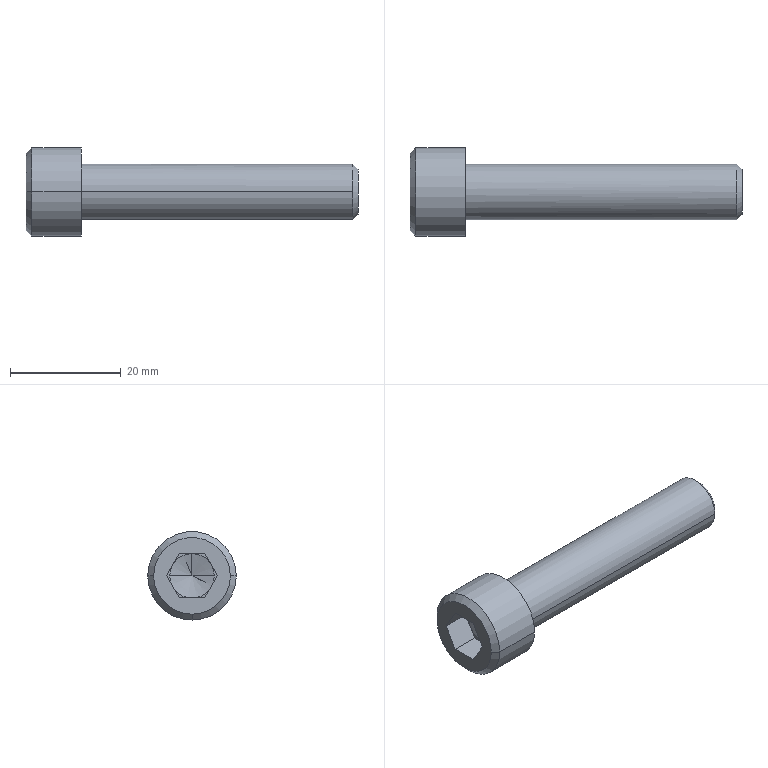Part | STEP file | 0244_307_SCB10-50 | 1 solid | 30 faces | box 60 x 16 x 16 mm | volume 5603 mm3 | plane 15 | cone 9 | cylinder 6 | commonest cylinder face diameters 10 x3 16 x3